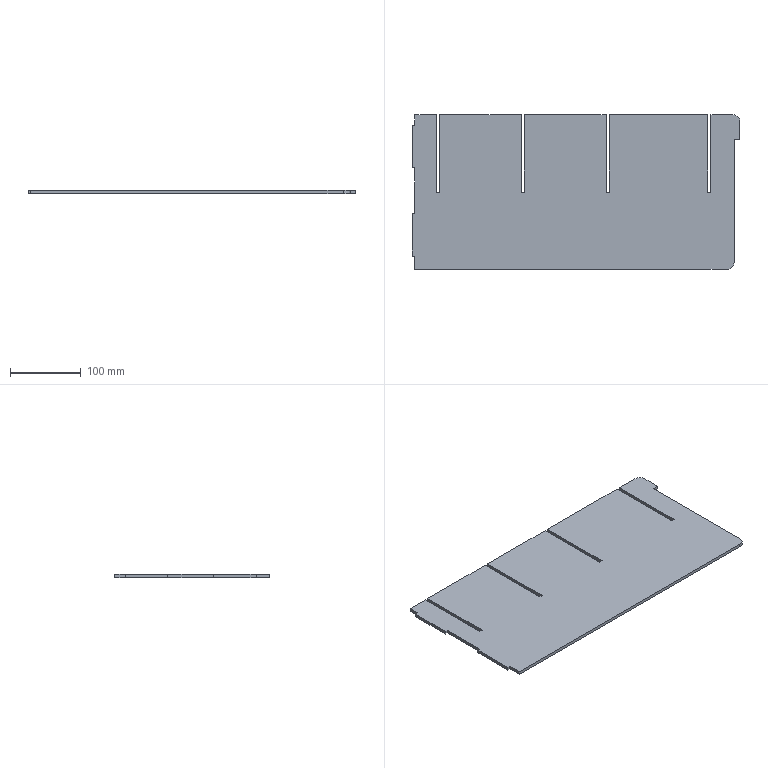Part | SolidWorks | features Fillet 1, FlatPattern 1, SMBaseFlange 1, SheetMetal 1 | 1 solid | 34 faces | box 464 x 218.7 x 4.5 mm | volume 438971 mm3 | plane 32 | cylinder 2 | commonest cylinder face diameters 20 x2
STEP:
#1=CARTESIAN_POINT('',(-230.,45.,0.));
#2=VERTEX_POINT('',#1);
#3=CARTESIAN_POINT('',(-230.,30.,0.));
#4=VERTEX_POINT('',#3);
#5=CARTESIAN_POINT('',(-230.,45.,0.));
#6=DIRECTION('',(0.,-1.,0.));
#7=VECTOR('',#6,1000.);
#8=LINE('',#5,#7);
#9=EDGE_CURVE('',#2,#4,#8,.T.);
#10=ORIENTED_EDGE('',*,*,#9,.T.);
#11=CARTESIAN_POINT('',(-230.,30.,4.5));
#12=VERTEX_POINT('',#11);
#13=CARTESIAN_POINT('',(-230.,30.,4.5));
#14=DIRECTION('',(0.,0.,-1.));
#15=VECTOR('',#14,1000.);
#16=LINE('',#13,#15);
#17=EDGE_CURVE('',#12,#4,#16,.T.);
#18=ORIENTED_EDGE('',*,*,#17,.F.);
#19=CARTESIAN_POINT('',(-230.,45.,4.5));
#20=VERTEX_POINT('',#19);
#21=CARTESIAN_POINT('',(-230.,45.,4.5));
#22=DIRECTION('',(0.,-1.,0.));
#23=VECTOR('',#22,1000.);
#24=LINE('',#21,#23);
#25=EDGE_CURVE('',#20,#12,#24,.T.);
#26=ORIENTED_EDGE('',*,*,#25,.F.);
#27=CARTESIAN_POINT('',(-230.,45.,4.5));
#28=DIRECTION('',(0.,0.,-1.));
#29=VECTOR('',#28,1000.);
#30=LINE('',#27,#29);
#31=EDGE_CURVE('',#20,#2,#30,.T.);
#32=ORIENTED_EDGE('',*,*,#31,.T.);
#33=EDGE_LOOP('',(#10,#18,#26,#32));
#34=FACE_OUTER_BOUND('',#33,.T.);
#35=CARTESIAN_POINT('',(-230.,45.,4.5));
#36=DIRECTION('',(1.,0.,0.));
#37=DIRECTION('',(0.,1.,0.));
#38=AXIS2_PLACEMENT_3D('',#35,#36,#37);
#39=PLANE('',#38);
#40=ADVANCED_FACE('',(#34),#39,.F.);
#41=CARTESIAN_POINT('',(-234.,30.,0.));
#42=VERTEX_POINT('',#41);
#43=CARTESIAN_POINT('',(-230.,30.,0.));
#44=DIRECTION('',(-1.,0.,0.));
#45=VECTOR('',#44,1000.);
#46=LINE('',#43,#45);
#47=EDGE_CURVE('',#4,#42,#46,.T.);
#48=ORIENTED_EDGE('',*,*,#47,.T.);
#49=CARTESIAN_POINT('',(-234.,30.,4.5));
#50=VERTEX_POINT('',#49);
#51=CARTESIAN_POINT('',(-234.,30.,4.5));
#52=DIRECTION('',(0.,0.,-1.));
#53=VECTOR('',#52,1000.);
#54=LINE('',#51,#53);
#55=EDGE_CURVE('',#50,#42,#54,.T.);
#56=ORIENTED_EDGE('',*,*,#55,.F.);
#57=CARTESIAN_POINT('',(-230.,30.,4.5));
#58=DIRECTION('',(-1.,0.,0.));
#59=VECTOR('',#58,1000.);
#60=LINE('',#57,#59);
#61=EDGE_CURVE('',#12,#50,#60,.T.);
#62=ORIENTED_EDGE('',*,*,#61,.F.);
#63=ORIENTED_EDGE('',*,*,#17,.T.);
#64=EDGE_LOOP('',(#48,#56,#62,#63));
#65=FACE_OUTER_BOUND('',#64,.T.);
#66=CARTESIAN_POINT('',(-230.,30.,4.5));
#67=DIRECTION('',(0.,-1.,0.));
#68=DIRECTION('',(0.,0.,-1.));
#69=AXIS2_PLACEMENT_3D('',#66,#67,#68);
#70=PLANE('',#69);
#71=ADVANCED_FACE('',(#65),#70,.F.);
#72=CARTESIAN_POINT('',(-234.,-30.,0.));
#73=VERTEX_POINT('',#72);
#74=CARTESIAN_POINT('',(-234.,30.,0.));
#75=DIRECTION('',(0.,-1.,0.));
#76=VECTOR('',#75,1000.);
#77=LINE('',#74,#76);
#78=EDGE_CURVE('',#42,#73,#77,.T.);
#79=ORIENTED_EDGE('',*,*,#78,.T.);
#80=CARTESIAN_POINT('',(-234.,-30.,4.5));
#81=VERTEX_POINT('',#80);
#82=CARTESIAN_POINT('',(-234.,-30.,4.5));
#83=DIRECTION('',(0.,0.,-1.));
#84=VECTOR('',#83,1000.);
#85=LINE('',#82,#84);
#86=EDGE_CURVE('',#81,#73,#85,.T.);
#87=ORIENTED_EDGE('',*,*,#86,.F.);
#88=CARTESIAN_POINT('',(-234.,30.,4.5));
#89=DIRECTION('',(0.,-1.,0.));
#90=VECTOR('',#89,1000.);
#91=LINE('',#88,#90);
#92=EDGE_CURVE('',#50,#81,#91,.T.);
#93=ORIENTED_EDGE('',*,*,#92,.F.);
#94=ORIENTED_EDGE('',*,*,#55,.T.);
#95=EDGE_LOOP('',(#79,#87,#93,#94));
#96=FACE_OUTER_BOUND('',#95,.T.);
#97=CARTESIAN_POINT('',(-234.,30.,4.5));
#98=DIRECTION('',(1.,0.,0.));
#99=DIRECTION('',(0.,0.,-1.));
#100=AXIS2_PLACEMENT_3D('',#97,#98,#99);
#101=PLANE('',#100);
#102=ADVANCED_FACE('',(#96),#101,.F.);
#103=CARTESIAN_POINT('',(-230.,-30.,0.));
#104=VERTEX_POINT('',#103);
#105=CARTESIAN_POINT('',(-234.,-30.,0.));
#106=DIRECTION('',(1.,0.,0.));
#107=VECTOR('',#106,1000.);
#108=LINE('',#105,#107);
#109=EDGE_CURVE('',#73,#104,#108,.T.);
#110=ORIENTED_EDGE('',*,*,#109,.T.);
#111=CARTESIAN_POINT('',(-230.,-30.,4.5));
#112=VERTEX_POINT('',#111);
#113=CARTESIAN_POINT('',(-230.,-30.,4.5));
#114=DIRECTION('',(0.,0.,-1.));
#115=VECTOR('',#114,1000.);
#116=LINE('',#113,#115);
#117=EDGE_CURVE('',#112,#104,#116,.T.);
#118=ORIENTED_EDGE('',*,*,#117,.F.);
#119=CARTESIAN_POINT('',(-234.,-30.,4.5));
#120=DIRECTION('',(1.,0.,0.));
#121=VECTOR('',#120,1000.);
#122=LINE('',#119,#121);
#123=EDGE_CURVE('',#81,#112,#122,.T.);
#124=ORIENTED_EDGE('',*,*,#123,.F.);
#125=ORIENTED_EDGE('',*,*,#86,.T.);
#126=EDGE_LOOP('',(#110,#118,#124,#125));
#127=FACE_OUTER_BOUND('',#126,.T.);
#128=CARTESIAN_POINT('',(-234.,-30.,4.5));
#129=DIRECTION('',(0.,1.,0.));
#130=DIRECTION('',(0.,0.,1.));
#131=AXIS2_PLACEMENT_3D('',#128,#129,#130);
#132=PLANE('',#131);
#133=ADVANCED_FACE('',(#127),#132,.F.);
#134=CARTESIAN_POINT('',(-230.,-95.,0.));
#135=VERTEX_POINT('',#134);
#136=CARTESIAN_POINT('',(-230.,-30.,0.));
#137=DIRECTION('',(0.,-1.,0.));
#138=VECTOR('',#137,1000.);
#139=LINE('',#136,#138);
#140=EDGE_CURVE('',#104,#135,#139,.T.);
#141=ORIENTED_EDGE('',*,*,#140,.T.);
#142=CARTESIAN_POINT('',(-230.,-95.,4.5));
#143=VERTEX_POINT('',#142);
#144=CARTESIAN_POINT('',(-230.,-95.,4.5));
#145=DIRECTION('',(0.,0.,-1.));
#146=VECTOR('',#145,1000.);
#147=LINE('',#144,#146);
#148=EDGE_CURVE('',#143,#135,#147,.T.);
#149=ORIENTED_EDGE('',*,*,#148,.F.);
#150=CARTESIAN_POINT('',(-230.,-30.,4.5));
#151=DIRECTION('',(0.,-1.,0.));
#152=VECTOR('',#151,1000.);
#153=LINE('',#150,#152);
#154=EDGE_CURVE('',#112,#143,#153,.T.);
#155=ORIENTED_EDGE('',*,*,#154,.F.);
#156=ORIENTED_EDGE('',*,*,#117,.T.);
#157=EDGE_LOOP('',(#141,#149,#155,#156));
#158=FACE_OUTER_BOUND('',#157,.T.);
#159=CARTESIAN_POINT('',(-230.,-30.,4.5));
#160=DIRECTION('',(1.,0.,0.));
#161=DIRECTION('',(0.,1.,0.));
#162=AXIS2_PLACEMENT_3D('',#159,#160,#161);
#163=PLANE('',#162);
#164=ADVANCED_FACE('',(#158),#163,.F.);
#165=CARTESIAN_POINT('',(-234.,-95.,0.));
#166=VERTEX_POINT('',#165);
#167=CARTESIAN_POINT('',(-234.,-95.,0.));
#168=DIRECTION('',(-1.,0.,0.));
#169=VECTOR('',#168,1000.);
#170=LINE('',#167,#169);
#171=EDGE_CURVE('',#135,#166,#170,.T.);
#172=ORIENTED_EDGE('',*,*,#171,.T.);
#173=CARTESIAN_POINT('',(-234.,-95.,4.5));
#174=VERTEX_POINT('',#173);
#175=CARTESIAN_POINT('',(-234.,-95.,4.5));
#176=DIRECTION('',(0.,0.,-1.));
#177=VECTOR('',#176,1000.);
#178=LINE('',#175,#177);
#179=EDGE_CURVE('',#174,#166,#178,.T.);
#180=ORIENTED_EDGE('',*,*,#179,.F.);
#181=CARTESIAN_POINT('',(-234.,-95.,4.5));
#182=DIRECTION('',(-1.,0.,0.));
#183=VECTOR('',#182,1000.);
#184=LINE('',#181,#183);
#185=EDGE_CURVE('',#143,#174,#184,.T.);
#186=ORIENTED_EDGE('',*,*,#185,.F.);
#187=ORIENTED_EDGE('',*,*,#148,.T.);
#188=EDGE_LOOP('',(#172,#180,#186,#187));
#189=FACE_OUTER_BOUND('',#188,.T.);
#190=CARTESIAN_POINT('',(-234.,-95.,4.5));
#191=DIRECTION('',(0.,-1.,0.));
#192=DIRECTION('',(0.,0.,-1.));
#193=AXIS2_PLACEMENT_3D('',#190,#191,#192);
#194=PLANE('',#193);
#195=ADVANCED_FACE('',(#189),#194,.F.);
#196=CARTESIAN_POINT('',(-234.,-155.,0.));
#197=VERTEX_POINT('',#196);
#198=CARTESIAN_POINT('',(-234.,-155.,0.));
#199=DIRECTION('',(0.,-1.,0.));
#200=VECTOR('',#199,1000.);
#201=LINE('',#198,#200);
#202=EDGE_CURVE('',#166,#197,#201,.T.);
#203=ORIENTED_EDGE('',*,*,#202,.T.);
#204=CARTESIAN_POINT('',(-234.,-155.,4.5));
#205=VERTEX_POINT('',#204);
#206=CARTESIAN_POINT('',(-234.,-155.,4.5));
#207=DIRECTION('',(0.,0.,-1.));
#208=VECTOR('',#207,1000.);
#209=LINE('',#206,#208);
#210=EDGE_CURVE('',#205,#197,#209,.T.);
#211=ORIENTED_EDGE('',*,*,#210,.F.);
#212=CARTESIAN_POINT('',(-234.,-155.,4.5));
#213=DIRECTION('',(0.,-1.,0.));
#214=VECTOR('',#213,1000.);
#215=LINE('',#212,#214);
#216=EDGE_CURVE('',#174,#205,#215,.T.);
#217=ORIENTED_EDGE('',*,*,#216,.F.);
#218=ORIENTED_EDGE('',*,*,#179,.T.);
#219=EDGE_LOOP('',(#203,#211,#217,#218));
#220=FACE_OUTER_BOUND('',#219,.T.);
#221=CARTESIAN_POINT('',(-234.,-155.,4.5));
#222=DIRECTION('',(1.,0.,0.));
#223=DIRECTION('',(0.,1.,0.));
#224=AXIS2_PLACEMENT_3D('',#221,#222,#223);
#225=PLANE('',#224);
#226=ADVANCED_FACE('',(#220),#225,.F.);
#227=CARTESIAN_POINT('',(-230.,-155.,0.));
#228=VERTEX_POINT('',#227);
#229=CARTESIAN_POINT('',(-230.,-155.,0.));
#230=DIRECTION('',(1.,0.,0.));
#231=VECTOR('',#230,1000.);
#232=LINE('',#229,#231);
#233=EDGE_CURVE('',#197,#228,#232,.T.);
#234=ORIENTED_EDGE('',*,*,#233,.T.);
#235=CARTESIAN_POINT('',(-230.,-155.,4.5));
#236=VERTEX_POINT('',#235);
#237=CARTESIAN_POINT('',(-230.,-155.,4.5));
#238=DIRECTION('',(0.,0.,-1.));
#239=VECTOR('',#238,1000.);
#240=LINE('',#237,#239);
#241=EDGE_CURVE('',#236,#228,#240,.T.);
#242=ORIENTED_EDGE('',*,*,#241,.F.);
#243=CARTESIAN_POINT('',(-230.,-155.,4.5));
#244=DIRECTION('',(1.,0.,0.));
#245=VECTOR('',#244,1000.);
#246=LINE('',#243,#245);
#247=EDGE_CURVE('',#205,#236,#246,.T.);
#248=ORIENTED_EDGE('',*,*,#247,.F.);
#249=ORIENTED_EDGE('',*,*,#210,.T.);
#250=EDGE_LOOP('',(#234,#242,#248,#249));
#251=FACE_OUTER_BOUND('',#250,.T.);
#252=CARTESIAN_POINT('',(-230.,-155.,4.5));
#253=DIRECTION('',(0.,1.,0.));
#254=DIRECTION('',(0.,0.,1.));
#255=AXIS2_PLACEMENT_3D('',#252,#253,#254);
#256=PLANE('',#255);
#257=ADVANCED_FACE('',(#251),#256,.F.);
#258=CARTESIAN_POINT('',(-230.,-173.7,0.));
#259=VERTEX_POINT('',#258);
#260=CARTESIAN_POINT('',(-230.,-155.,0.));
#261=DIRECTION('',(0.,-1.,0.));
#262=VECTOR('',#261,1000.);
#263=LINE('',#260,#262);
#264=EDGE_CURVE('',#228,#259,#263,.T.);
#265=ORIENTED_EDGE('',*,*,#264,.T.);
#266=CARTESIAN_POINT('',(-230.,-173.7,4.5));
#267=VERTEX_POINT('',#266);
#268=CARTESIAN_POINT('',(-230.,-173.7,4.5));
#269=DIRECTION('',(0.,0.,-1.));
#270=VECTOR('',#269,1000.);
#271=LINE('',#268,#270);
#272=EDGE_CURVE('',#267,#259,#271,.T.);
#273=ORIENTED_EDGE('',*,*,#272,.F.);
#274=CARTESIAN_POINT('',(-230.,-155.,4.5));
#275=DIRECTION('',(0.,-1.,0.));
#276=VECTOR('',#275,1000.);
#277=LINE('',#274,#276);
#278=EDGE_CURVE('',#236,#267,#277,.T.);
#279=ORIENTED_EDGE('',*,*,#278,.F.);
#280=ORIENTED_EDGE('',*,*,#241,.T.);
#281=EDGE_LOOP('',(#265,#273,#279,#280));
#282=FACE_OUTER_BOUND('',#281,.T.);
#283=CARTESIAN_POINT('',(-230.,-155.,4.5));
#284=DIRECTION('',(1.,0.,0.));
#285=DIRECTION('',(0.,1.,0.));
#286=AXIS2_PLACEMENT_3D('',#283,#284,#285);
#287=PLANE('',#286);
#288=ADVANCED_FACE('',(#282),#287,.F.);
#289=CARTESIAN_POINT('',(211.7,-173.7,0.));
#290=VERTEX_POINT('',#289);
#291=CARTESIAN_POINT('',(-230.,-173.7,0.));
#292=DIRECTION('',(1.,0.,0.));
#293=VECTOR('',#292,1000.);
#294=LINE('',#291,#293);
#295=EDGE_CURVE('',#259,#290,#294,.T.);
#296=ORIENTED_EDGE('',*,*,#295,.T.);
#297=CARTESIAN_POINT('',(211.7,-173.7,4.5));
#298=VERTEX_POINT('',#297);
#299=CARTESIAN_POINT('',(211.7,-173.7,4.5));
#300=DIRECTION('',(0.,0.,1.));
#301=VECTOR('',#300,1000.);
#302=LINE('',#299,#301);
#303=EDGE_CURVE('',#290,#298,#302,.T.);
#304=ORIENTED_EDGE('',*,*,#303,.T.);
#305=CARTESIAN_POINT('',(-230.,-173.7,4.5));
#306=DIRECTION('',(1.,0.,0.));
#307=VECTOR('',#306,1000.);
#308=LINE('',#305,#307);
#309=EDGE_CURVE('',#267,#298,#308,.T.);
#310=ORIENTED_EDGE('',*,*,#309,.F.);
#311=ORIENTED_EDGE('',*,*,#272,.T.);
#312=EDGE_LOOP('',(#296,#304,#310,#311));
#313=FACE_OUTER_BOUND('',#312,.T.);
#314=CARTESIAN_POINT('',(-230.,-173.7,4.5));
#315=DIRECTION('',(0.,1.,0.));
#316=DIRECTION('',(0.,0.,1.));
#317=AXIS2_PLACEMENT_3D('',#314,#315,#316);
#318=PLANE('',#317);
#319=ADVANCED_FACE('',(#313),#318,.F.);
#320=CARTESIAN_POINT('',(221.7,-163.7,4.5));
#321=VERTEX_POINT('',#320);
#322=CARTESIAN_POINT('',(221.7,9.3,4.5));
#323=VERTEX_POINT('',#322);
#324=CARTESIAN_POINT('',(221.7,9.3,4.5));
#325=DIRECTION('',(0.,1.,0.));
#326=VECTOR('',#325,1000.);
#327=LINE('',#324,#326);
#328=EDGE_CURVE('',#321,#323,#327,.T.);
#329=ORIENTED_EDGE('',*,*,#328,.F.);
#330=CARTESIAN_POINT('',(221.7,-163.7,0.));
#331=VERTEX_POINT('',#330);
#332=CARTESIAN_POINT('',(221.7,-163.7,4.5));
#333=DIRECTION('',(0.,0.,-1.));
#334=VECTOR('',#333,1000.);
#335=LINE('',#332,#334);
#336=EDGE_CURVE('',#321,#331,#335,.T.);
#337=ORIENTED_EDGE('',*,*,#336,.T.);
#338=CARTESIAN_POINT('',(221.7,9.3,0.));
#339=VERTEX_POINT('',#338);
#340=CARTESIAN_POINT('',(221.7,9.3,0.));
#341=DIRECTION('',(0.,1.,0.));
#342=VECTOR('',#341,1000.);
#343=LINE('',#340,#342);
#344=EDGE_CURVE('',#331,#339,#343,.T.);
#345=ORIENTED_EDGE('',*,*,#344,.T.);
#346=CARTESIAN_POINT('',(221.7,9.3,4.5));
#347=DIRECTION('',(0.,0.,-1.));
#348=VECTOR('',#347,1000.);
#349=LINE('',#346,#348);
#350=EDGE_CURVE('',#323,#339,#349,.T.);
#351=ORIENTED_EDGE('',*,*,#350,.F.);
#352=EDGE_LOOP('',(#329,#337,#345,#351));
#353=FACE_OUTER_BOUND('',#352,.T.);
#354=CARTESIAN_POINT('',(221.7,9.3,4.5));
#355=DIRECTION('',(-1.,0.,0.));
#356=DIRECTION('',(0.,-1.,0.));
#357=AXIS2_PLACEMENT_3D('',#354,#355,#356);
#358=PLANE('',#357);
#359=ADVANCED_FACE('',(#353),#358,.F.);
#360=CARTESIAN_POINT('',(230.,9.3,0.));
#361=VERTEX_POINT('',#360);
#362=CARTESIAN_POINT('',(221.7,9.3,0.));
#363=DIRECTION('',(1.,0.,0.));
#364=VECTOR('',#363,1000.);
#365=LINE('',#362,#364);
#366=EDGE_CURVE('',#339,#361,#365,.T.);
#367=ORIENTED_EDGE('',*,*,#366,.T.);
#368=CARTESIAN_POINT('',(230.,9.3,4.5));
#369=VERTEX_POINT('',#368);
#370=CARTESIAN_POINT('',(230.,9.3,4.5));
#371=DIRECTION('',(0.,0.,-1.));
#372=VECTOR('',#371,1000.);
#373=LINE('',#370,#372);
#374=EDGE_CURVE('',#369,#361,#373,.T.);
#375=ORIENTED_EDGE('',*,*,#374,.F.);
#376=CARTESIAN_POINT('',(221.7,9.3,4.5));
#377=DIRECTION('',(1.,0.,0.));
#378=VECTOR('',#377,1000.);
#379=LINE('',#376,#378);
#380=EDGE_CURVE('',#323,#369,#379,.T.);
#381=ORIENTED_EDGE('',*,*,#380,.F.);
#382=ORIENTED_EDGE('',*,*,#350,.T.);
#383=EDGE_LOOP('',(#367,#375,#381,#382));
#384=FACE_OUTER_BOUND('',#383,.T.);
#385=CARTESIAN_POINT('',(221.7,9.3,4.5));
#386=DIRECTION('',(0.,1.,0.));
#387=DIRECTION('',(0.,0.,1.));
#388=AXIS2_PLACEMENT_3D('',#385,#386,#387);
#389=PLANE('',#388);
#390=ADVANCED_FACE('',(#384),#389,.F.);
#391=CARTESIAN_POINT('',(230.,35.,0.));
#392=VERTEX_POINT('',#391);
#393=CARTESIAN_POINT('',(230.,9.3,0.));
#394=DIRECTION('',(0.,1.,0.));
#395=VECTOR('',#394,1000.);
#396=LINE('',#393,#395);
#397=EDGE_CURVE('',#361,#392,#396,.T.);
#398=ORIENTED_EDGE('',*,*,#397,.T.);
#399=CARTESIAN_POINT('',(230.,35.,4.5));
#400=VERTEX_POINT('',#399);
#401=CARTESIAN_POINT('',(230.,35.,4.5));
#402=DIRECTION('',(0.,0.,1.));
#403=VECTOR('',#402,1000.);
#404=LINE('',#401,#403);
#405=EDGE_CURVE('',#392,#400,#404,.T.);
#406=ORIENTED_EDGE('',*,*,#405,.T.);
#407=CARTESIAN_POINT('',(230.,9.3,4.5));
#408=DIRECTION('',(0.,1.,0.));
#409=VECTOR('',#408,1000.);
#410=LINE('',#407,#409);
#411=EDGE_CURVE('',#369,#400,#410,.T.);
#412=ORIENTED_EDGE('',*,*,#411,.F.);
#413=ORIENTED_EDGE('',*,*,#374,.T.);
#414=EDGE_LOOP('',(#398,#406,#412,#413));
#415=FACE_OUTER_BOUND('',#414,.T.);
#416=CARTESIAN_POINT('',(230.,9.3,4.5));
#417=DIRECTION('',(-1.,0.,0.));
#418=DIRECTION('',(0.,-1.,0.));
#419=AXIS2_PLACEMENT_3D('',#416,#417,#418);
#420=PLANE('',#419);
#421=ADVANCED_FACE('',(#415),#420,.F.);
#422=CARTESIAN_POINT('',(220.,45.,4.5));
#423=VERTEX_POINT('',#422);
#424=CARTESIAN_POINT('',(189.,45.,4.5));
#425=VERTEX_POINT('',#424);
#426=CARTESIAN_POINT('',(189.,45.,4.5));
#427=DIRECTION('',(-1.,0.,0.));
#428=VECTOR('',#427,1000.);
#429=LINE('',#426,#428);
#430=EDGE_CURVE('',#423,#425,#429,.T.);
#431=ORIENTED_EDGE('',*,*,#430,.F.);
#432=CARTESIAN_POINT('',(220.,45.,0.));
#433=VERTEX_POINT('',#432);
#434=CARTESIAN_POINT('',(220.,45.,4.5));
#435=DIRECTION('',(0.,0.,-1.));
#436=VECTOR('',#435,1000.);
#437=LINE('',#434,#436);
#438=EDGE_CURVE('',#423,#433,#437,.T.);
#439=ORIENTED_EDGE('',*,*,#438,.T.);
#440=CARTESIAN_POINT('',(189.,45.,0.));
#441=VERTEX_POINT('',#440);
#442=CARTESIAN_POINT('',(189.,45.,0.));
#443=DIRECTION('',(-1.,0.,0.));
#444=VECTOR('',#443,1000.);
#445=LINE('',#442,#444);
#446=EDGE_CURVE('',#433,#441,#445,.T.);
#447=ORIENTED_EDGE('',*,*,#446,.T.);
#448=CARTESIAN_POINT('',(189.,45.,4.5));
#449=DIRECTION('',(0.,0.,-1.));
#450=VECTOR('',#449,1000.);
#451=LINE('',#448,#450);
#452=EDGE_CURVE('',#425,#441,#451,.T.);
#453=ORIENTED_EDGE('',*,*,#452,.F.);
#454=EDGE_LOOP('',(#431,#439,#447,#453));
#455=FACE_OUTER_BOUND('',#454,.T.);
#456=CARTESIAN_POINT('',(189.,45.,4.5));
#457=DIRECTION('',(0.,-1.,0.));
#458=DIRECTION('',(1.,0.,0.));
#459=AXIS2_PLACEMENT_3D('',#456,#457,#458);
#460=PLANE('',#459);
#461=ADVANCED_FACE('',(#455),#460,.F.);
#462=CARTESIAN_POINT('',(189.,-64.5,0.));
#463=VERTEX_POINT('',#462);
#464=CARTESIAN_POINT('',(189.,45.,0.));
#465=DIRECTION('',(0.,-1.,0.));
#466=VECTOR('',#465,1000.);
#467=LINE('',#464,#466);
#468=EDGE_CURVE('',#441,#463,#467,.T.);
#469=ORIENTED_EDGE('',*,*,#468,.T.);
#470=CARTESIAN_POINT('',(189.,-64.5,4.5));
#471=VERTEX_POINT('',#470);
#472=CARTESIAN_POINT('',(189.,-64.5,4.5));
#473=DIRECTION('',(0.,0.,-1.));
#474=VECTOR('',#473,1000.);
#475=LINE('',#472,#474);
#476=EDGE_CURVE('',#471,#463,#475,.T.);
#477=ORIENTED_EDGE('',*,*,#476,.F.);
#478=CARTESIAN_POINT('',(189.,45.,4.5));
#479=DIRECTION('',(0.,-1.,0.));
#480=VECTOR('',#479,1000.);
#481=LINE('',#478,#480);
#482=EDGE_CURVE('',#425,#471,#481,.T.);
#483=ORIENTED_EDGE('',*,*,#482,.F.);
#484=ORIENTED_EDGE('',*,*,#452,.T.);
#485=EDGE_LOOP('',(#469,#477,#483,#484));
#486=FACE_OUTER_BOUND('',#485,.T.);
#487=CARTESIAN_POINT('',(189.,45.,4.5));
#488=DIRECTION('',(1.,0.,0.));
#489=DIRECTION('',(0.,1.,0.));
#490=AXIS2_PLACEMENT_3D('',#487,#488,#489);
#491=PLANE('',#490);
#492=ADVANCED_FACE('',(#486),#491,.F.);
#493=CARTESIAN_POINT('',(184.5,-64.5,0.));
#494=VERTEX_POINT('',#493);
#495=CARTESIAN_POINT('',(189.,-64.5,0.));
#496=DIRECTION('',(-1.,0.,0.));
#497=VECTOR('',#496,1000.);
#498=LINE('',#495,#497);
#499=EDGE_CURVE('',#463,#494,#498,.T.);
#500=ORIENTED_EDGE('',*,*,#499,.T.);
#501=CARTESIAN_POINT('',(184.5,-64.5,4.5));
#502=VERTEX_POINT('',#501);
#503=CARTESIAN_POINT('',(184.5,-64.5,4.5));
#504=DIRECTION('',(0.,0.,-1.));
#505=VECTOR('',#504,1000.);
#506=LINE('',#503,#505);
#507=EDGE_CURVE('',#502,#494,#506,.T.);
#508=ORIENTED_EDGE('',*,*,#507,.F.);
#509=CARTESIAN_POINT('',(189.,-64.5,4.5));
#510=DIRECTION('',(-1.,0.,0.));
#511=VECTOR('',#510,1000.);
#512=LINE('',#509,#511);
#513=EDGE_CURVE('',#471,#502,#512,.T.);
#514=ORIENTED_EDGE('',*,*,#513,.F.);
#515=ORIENTED_EDGE('',*,*,#476,.T.);
#516=EDGE_LOOP('',(#500,#508,#514,#515));
#517=FACE_OUTER_BOUND('',#516,.T.);
#518=CARTESIAN_POINT('',(189.,-64.5,4.5));
#519=DIRECTION('',(0.,-1.,0.));
#520=DIRECTION('',(1.,0.,0.));
#521=AXIS2_PLACEMENT_3D('',#518,#519,#520);
#522=PLANE('',#521);
#523=ADVANCED_FACE('',(#517),#522,.F.);
#524=CARTESIAN_POINT('',(184.5,45.,0.));
#525=VERTEX_POINT('',#524);
#526=CARTESIAN_POINT('',(184.5,-64.5,0.));
#527=DIRECTION('',(0.,1.,0.));
#528=VECTOR('',#527,1000.);
#529=LINE('',#526,#528);
#530=EDGE_CURVE('',#494,#525,#529,.T.);
#531=ORIENTED_EDGE('',*,*,#530,.T.);
#532=CARTESIAN_POINT('',(184.5,45.,4.5));
#533=VERTEX_POINT('',#532);
#534=CARTESIAN_POINT('',(184.5,45.,4.5));
#535=DIRECTION('',(0.,0.,-1.));
#536=VECTOR('',#535,1000.);
#537=LINE('',#534,#536);
#538=EDGE_CURVE('',#533,#525,#537,.T.);
#539=ORIENTED_EDGE('',*,*,#538,.F.);
#540=CARTESIAN_POINT('',(184.5,-64.5,4.5));
#541=DIRECTION('',(0.,1.,0.));
#542=VECTOR('',#541,1000.);
#543=LINE('',#540,#542);
#544=EDGE_CURVE('',#502,#533,#543,.T.);
#545=ORIENTED_EDGE('',*,*,#544,.F.);
#546=ORIENTED_EDGE('',*,*,#507,.T.);
#547=EDGE_LOOP('',(#531,#539,#545,#546));
#548=FACE_OUTER_BOUND('',#547,.T.);
#549=CARTESIAN_POINT('',(184.5,-64.5,4.5));
#550=DIRECTION('',(-1.,0.,0.));
#551=DIRECTION('',(0.,-1.,0.));
#552=AXIS2_PLACEMENT_3D('',#549,#550,#551);
#553=PLANE('',#552);
#554=ADVANCED_FACE('',(#548),#553,.F.);
#555=CARTESIAN_POINT('',(45.,45.,0.));
#556=VERTEX_POINT('',#555);
#557=CARTESIAN_POINT('',(45.,45.,0.));
#558=DIRECTION('',(-1.,0.,0.));
#559=VECTOR('',#558,1000.);
#560=LINE('',#557,#559);
#561=EDGE_CURVE('',#525,#556,#560,.T.);
#562=ORIENTED_EDGE('',*,*,#561,.T.);
#563=CARTESIAN_POINT('',(45.,45.,4.5));
#564=VERTEX_POINT('',#563);
#565=CARTESIAN_POINT('',(45.,45.,4.5));
#566=DIRECTION('',(0.,0.,-1.));
#567=VECTOR('',#566,1000.);
#568=LINE('',#565,#567);
#569=EDGE_CURVE('',#564,#556,#568,.T.);
#570=ORIENTED_EDGE('',*,*,#569,.F.);
#571=CARTESIAN_POINT('',(45.,45.,4.5));
#572=DIRECTION('',(-1.,0.,0.));
#573=VECTOR('',#572,1000.);
#574=LINE('',#571,#573);
#575=EDGE_CURVE('',#533,#564,#574,.T.);
#576=ORIENTED_EDGE('',*,*,#575,.F.);
#577=ORIENTED_EDGE('',*,*,#538,.T.);
#578=EDGE_LOOP('',(#562,#570,#576,#577));
#579=FACE_OUTER_BOUND('',#578,.T.);
#580=CARTESIAN_POINT('',(45.,45.,4.5));
#581=DIRECTION('',(0.,-1.,0.));
#582=DIRECTION('',(1.,0.,0.));
#583=AXIS2_PLACEMENT_3D('',#580,#581,#582);
#584=PLANE('',#583);
#585=ADVANCED_FACE('',(#579),#584,.F.);
#586=CARTESIAN_POINT('',(45.,-64.5,0.));
#587=VERTEX_POINT('',#586);
#588=CARTESIAN_POINT('',(45.,45.,0.));
#589=DIRECTION('',(0.,-1.,0.));
#590=VECTOR('',#589,1000.);
#591=LINE('',#588,#590);
#592=EDGE_CURVE('',#556,#587,#591,.T.);
#593=ORIENTED_EDGE('',*,*,#592,.T.);
#594=CARTESIAN_POINT('',(45.,-64.5,4.5));
#595=VERTEX_POINT('',#594);
#596=CARTESIAN_POINT('',(45.,-64.5,4.5));
#597=DIRECTION('',(0.,0.,-1.));
#598=VECTOR('',#597,1000.);
#599=LINE('',#596,#598);
#600=EDGE_CURVE('',#595,#587,#599,.T.);
#601=ORIENTED_EDGE('',*,*,#600,.F.);
#602=CARTESIAN_POINT('',(45.,45.,4.5));
#603=DIRECTION('',(0.,-1.,0.));
#604=VECTOR('',#603,1000.);
#605=LINE('',#602,#604);
#606=EDGE_CURVE('',#564,#595,#605,.T.);
#607=ORIENTED_EDGE('',*,*,#606,.F.);
#608=ORIENTED_EDGE('',*,*,#569,.T.);
#609=EDGE_LOOP('',(#593,#601,#607,#608));
#610=FACE_OUTER_BOUND('',#609,.T.);
#611=CARTESIAN_POINT('',(45.,45.,4.5));
#612=DIRECTION('',(1.,0.,0.));
#613=DIRECTION('',(0.,1.,0.));
#614=AXIS2_PLACEMENT_3D('',#611,#612,#613);
#615=PLANE('',#614);
#616=ADVANCED_FACE('',(#610),#615,.F.);
#617=CARTESIAN_POINT('',(40.5,-64.5,0.));
#618=VERTEX_POINT('',#617);
#619=CARTESIAN_POINT('',(45.,-64.5,0.));
#620=DIRECTION('',(-1.,0.,0.));
#621=VECTOR('',#620,1000.);
#622=LINE('',#619,#621);
#623=EDGE_CURVE('',#587,#618,#622,.T.);
#624=ORIENTED_EDGE('',*,*,#623,.T.);
#625=CARTESIAN_POINT('',(40.5,-64.5,4.5));
#626=VERTEX_POINT('',#625);
#627=CARTESIAN_POINT('',(40.5,-64.5,4.5));
#628=DIRECTION('',(0.,0.,-1.));
#629=VECTOR('',#628,1000.);
#630=LINE('',#627,#629);
#631=EDGE_CURVE('',#626,#618,#630,.T.);
#632=ORIENTED_EDGE('',*,*,#631,.F.);
#633=CARTESIAN_POINT('',(45.,-64.5,4.5));
#634=DIRECTION('',(-1.,0.,0.));
#635=VECTOR('',#634,1000.);
#636=LINE('',#633,#635);
#637=EDGE_CURVE('',#595,#626,#636,.T.);
#638=ORIENTED_EDGE('',*,*,#637,.F.);
#639=ORIENTED_EDGE('',*,*,#600,.T.);
#640=EDGE_LOOP('',(#624,#632,#638,#639));
#641=FACE_OUTER_BOUND('',#640,.T.);
#642=CARTESIAN_POINT('',(45.,-64.5,4.5));
#643=DIRECTION('',(0.,-1.,0.));
#644=DIRECTION('',(0.,0.,-1.));
#645=AXIS2_PLACEMENT_3D('',#642,#643,#644);
#646=PLANE('',#645);
#647=ADVANCED_FACE('',(#641),#646,.F.);
#648=CARTESIAN_POINT('',(40.5,45.,0.));
#649=VERTEX_POINT('',#648);
#650=CARTESIAN_POINT('',(40.5,-64.5,0.));
#651=DIRECTION('',(0.,1.,0.));
#652=VECTOR('',#651,1000.);
#653=LINE('',#650,#652);
#654=EDGE_CURVE('',#618,#649,#653,.T.);
#655=ORIENTED_EDGE('',*,*,#654,.T.);
#656=CARTESIAN_POINT('',(40.5,45.,4.5));
#657=VERTEX_POINT('',#656);
#658=CARTESIAN_POINT('',(40.5,45.,4.5));
#659=DIRECTION('',(0.,0.,-1.));
#660=VECTOR('',#659,1000.);
#661=LINE('',#658,#660);
#662=EDGE_CURVE('',#657,#649,#661,.T.);
#663=ORIENTED_EDGE('',*,*,#662,.F.);
#664=CARTESIAN_POINT('',(40.5,-64.5,4.5));
#665=DIRECTION('',(0.,1.,0.));
#666=VECTOR('',#665,1000.);
#667=LINE('',#664,#666);
#668=EDGE_CURVE('',#626,#657,#667,.T.);
#669=ORIENTED_EDGE('',*,*,#668,.F.);
#670=ORIENTED_EDGE('',*,*,#631,.T.);
#671=EDGE_LOOP('',(#655,#663,#669,#670));
#672=FACE_OUTER_BOUND('',#671,.T.);
#673=CARTESIAN_POINT('',(40.5,-64.5,4.5));
#674=DIRECTION('',(-1.,0.,0.));
#675=DIRECTION('',(0.,0.,1.));
#676=AXIS2_PLACEMENT_3D('',#673,#674,#675);
#677=PLANE('',#676);
#678=ADVANCED_FACE('',(#672),#677,.F.);
#679=CARTESIAN_POINT('',(-75.,45.,0.));
#680=VERTEX_POINT('',#679);
#681=CARTESIAN_POINT('',(-75.,45.,0.));
#682=DIRECTION('',(-1.,0.,0.));
#683=VECTOR('',#682,1000.);
#684=LINE('',#681,#683);
#685=EDGE_CURVE('',#649,#680,#684,.T.);
#686=ORIENTED_EDGE('',*,*,#685,.T.);
#687=CARTESIAN_POINT('',(-75.,45.,4.5));
#688=VERTEX_POINT('',#687);
#689=CARTESIAN_POINT('',(-75.,45.,4.5));
#690=DIRECTION('',(0.,0.,-1.));
#691=VECTOR('',#690,1000.);
#692=LINE('',#689,#691);
#693=EDGE_CURVE('',#688,#680,#692,.T.);
#694=ORIENTED_EDGE('',*,*,#693,.F.);
#695=CARTESIAN_POINT('',(-75.,45.,4.5));
#696=DIRECTION('',(-1.,0.,0.));
#697=VECTOR('',#696,1000.);
#698=LINE('',#695,#697);
#699=EDGE_CURVE('',#657,#688,#698,.T.);
#700=ORIENTED_EDGE('',*,*,#699,.F.);
#701=ORIENTED_EDGE('',*,*,#662,.T.);
#702=EDGE_LOOP('',(#686,#694,#700,#701));
#703=FACE_OUTER_BOUND('',#702,.T.);
#704=CARTESIAN_POINT('',(-75.,45.,4.5));
#705=DIRECTION('',(0.,-1.,0.));
#706=DIRECTION('',(1.,0.,0.));
#707=AXIS2_PLACEMENT_3D('',#704,#705,#706);
#708=PLANE('',#707);
#709=ADVANCED_FACE('',(#703),#708,.F.);
#710=CARTESIAN_POINT('',(-75.,-64.5,0.));
#711=VERTEX_POINT('',#710);
#712=CARTESIAN_POINT('',(-75.,45.,0.));
#713=DIRECTION('',(0.,-1.,0.));
#714=VECTOR('',#713,1000.);
#715=LINE('',#712,#714);
#716=EDGE_CURVE('',#680,#711,#715,.T.);
#717=ORIENTED_EDGE('',*,*,#716,.T.);
#718=CARTESIAN_POINT('',(-75.,-64.5,4.5));
#719=VERTEX_POINT('',#718);
#720=CARTESIAN_POINT('',(-75.,-64.5,4.5));
#721=DIRECTION('',(0.,0.,-1.));
#722=VECTOR('',#721,1000.);
#723=LINE('',#720,#722);
#724=EDGE_CURVE('',#719,#711,#723,.T.);
#725=ORIENTED_EDGE('',*,*,#724,.F.);
#726=CARTESIAN_POINT('',(-75.,45.,4.5));
#727=DIRECTION('',(0.,-1.,0.));
#728=VECTOR('',#727,1000.);
#729=LINE('',#726,#728);
#730=EDGE_CURVE('',#688,#719,#729,.T.);
#731=ORIENTED_EDGE('',*,*,#730,.F.);
#732=ORIENTED_EDGE('',*,*,#693,.T.);
#733=EDGE_LOOP('',(#717,#725,#731,#732));
#734=FACE_OUTER_BOUND('',#733,.T.);
#735=CARTESIAN_POINT('',(-75.,45.,4.5));
#736=DIRECTION('',(1.,0.,0.));
#737=DIRECTION('',(0.,1.,0.));
#738=AXIS2_PLACEMENT_3D('',#735,#736,#737);
#739=PLANE('',#738);
#740=ADVANCED_FACE('',(#734),#739,.F.);
#741=CARTESIAN_POINT('',(-79.5,-64.5,0.));
#742=VERTEX_POINT('',#741);
#743=CARTESIAN_POINT('',(-75.,-64.5,0.));
#744=DIRECTION('',(-1.,0.,0.));
#745=VECTOR('',#744,1000.);
#746=LINE('',#743,#745);
#747=EDGE_CURVE('',#711,#742,#746,.T.);
#748=ORIENTED_EDGE('',*,*,#747,.T.);
#749=CARTESIAN_POINT('',(-79.5,-64.5,4.5));
#750=VERTEX_POINT('',#749);
#751=CARTESIAN_POINT('',(-79.5,-64.5,4.5));
#752=DIRECTION('',(0.,0.,-1.));
#753=VECTOR('',#752,1000.);
#754=LINE('',#751,#753);
#755=EDGE_CURVE('',#750,#742,#754,.T.);
#756=ORIENTED_EDGE('',*,*,#755,.F.);
#757=CARTESIAN_POINT('',(-75.,-64.5,4.5));
#758=DIRECTION('',(-1.,0.,0.));
#759=VECTOR('',#758,1000.);
#760=LINE('',#757,#759);
#761=EDGE_CURVE('',#719,#750,#760,.T.);
#762=ORIENTED_EDGE('',*,*,#761,.F.);
#763=ORIENTED_EDGE('',*,*,#724,.T.);
#764=EDGE_LOOP('',(#748,#756,#762,#763));
#765=FACE_OUTER_BOUND('',#764,.T.);
#766=CARTESIAN_POINT('',(-75.,-64.5,4.5));
#767=DIRECTION('',(0.,-1.,0.));
#768=DIRECTION('',(0.,0.,-1.));
#769=AXIS2_PLACEMENT_3D('',#766,#767,#768);
#770=PLANE('',#769);
#771=ADVANCED_FACE('',(#765),#770,.F.);
#772=CARTESIAN_POINT('',(-79.5,45.,0.));
#773=VERTEX_POINT('',#772);
#774=CARTESIAN_POINT('',(-79.5,-64.5,0.));
#775=DIRECTION('',(0.,1.,0.));
#776=VECTOR('',#775,1000.);
#777=LINE('',#774,#776);
#778=EDGE_CURVE('',#742,#773,#777,.T.);
#779=ORIENTED_EDGE('',*,*,#778,.T.);
#780=CARTESIAN_POINT('',(-79.5,45.,4.5));
#781=VERTEX_POINT('',#780);
#782=CARTESIAN_POINT('',(-79.5,45.,4.5));
#783=DIRECTION('',(0.,0.,-1.));
#784=VECTOR('',#783,1000.);
#785=LINE('',#782,#784);
#786=EDGE_CURVE('',#781,#773,#785,.T.);
#787=ORIENTED_EDGE('',*,*,#786,.F.);
#788=CARTESIAN_POINT('',(-79.5,-64.5,4.5));
#789=DIRECTION('',(0.,1.,0.));
#790=VECTOR('',#789,1000.);
#791=LINE('',#788,#790);
#792=EDGE_CURVE('',#750,#781,#791,.T.);
#793=ORIENTED_EDGE('',*,*,#792,.F.);
#794=ORIENTED_EDGE('',*,*,#755,.T.);
#795=EDGE_LOOP('',(#779,#787,#793,#794));
#796=FACE_OUTER_BOUND('',#795,.T.);
#797=CARTESIAN_POINT('',(-79.5,-64.5,4.5));
#798=DIRECTION('',(-1.,0.,0.));
#799=DIRECTION('',(0.,0.,1.));
#800=AXIS2_PLACEMENT_3D('',#797,#798,#799);
#801=PLANE('',#800);
#802=ADVANCED_FACE('',(#796),#801,.F.);
#803=CARTESIAN_POINT('',(-195.,45.,0.));
#804=VERTEX_POINT('',#803);
#805=CARTESIAN_POINT('',(-195.,45.,0.));
#806=DIRECTION('',(-1.,0.,0.));
#807=VECTOR('',#806,1000.);
#808=LINE('',#805,#807);
#809=EDGE_CURVE('',#773,#804,#808,.T.);
#810=ORIENTED_EDGE('',*,*,#809,.T.);
#811=CARTESIAN_POINT('',(-195.,45.,4.5));
#812=VERTEX_POINT('',#811);
#813=CARTESIAN_POINT('',(-195.,45.,4.5));
#814=DIRECTION('',(0.,0.,-1.));
#815=VECTOR('',#814,1000.);
#816=LINE('',#813,#815);
#817=EDGE_CURVE('',#812,#804,#816,.T.);
#818=ORIENTED_EDGE('',*,*,#817,.F.);
#819=CARTESIAN_POINT('',(-195.,45.,4.5));
#820=DIRECTION('',(-1.,0.,0.));
#821=VECTOR('',#820,1000.);
#822=LINE('',#819,#821);
#823=EDGE_CURVE('',#781,#812,#822,.T.);
#824=ORIENTED_EDGE('',*,*,#823,.F.);
#825=ORIENTED_EDGE('',*,*,#786,.T.);
#826=EDGE_LOOP('',(#810,#818,#824,#825));
#827=FACE_OUTER_BOUND('',#826,.T.);
#828=CARTESIAN_POINT('',(-195.,45.,4.5));
#829=DIRECTION('',(0.,-1.,0.));
#830=DIRECTION('',(1.,0.,0.));
#831=AXIS2_PLACEMENT_3D('',#828,#829,#830);
#832=PLANE('',#831);
#833=ADVANCED_FACE('',(#827),#832,.F.);
#834=CARTESIAN_POINT('',(-195.,-64.5,0.));
#835=VERTEX_POINT('',#834);
#836=CARTESIAN_POINT('',(-195.,45.,0.));
#837=DIRECTION('',(0.,-1.,0.));
#838=VECTOR('',#837,1000.);
#839=LINE('',#836,#838);
#840=EDGE_CURVE('',#804,#835,#839,.T.);
#841=ORIENTED_EDGE('',*,*,#840,.T.);
#842=CARTESIAN_POINT('',(-195.,-64.5,4.5));
#843=VERTEX_POINT('',#842);
#844=CARTESIAN_POINT('',(-195.,-64.5,4.5));
#845=DIRECTION('',(0.,0.,-1.));
#846=VECTOR('',#845,1000.);
#847=LINE('',#844,#846);
#848=EDGE_CURVE('',#843,#835,#847,.T.);
#849=ORIENTED_EDGE('',*,*,#848,.F.);
#850=CARTESIAN_POINT('',(-195.,45.,4.5));
#851=DIRECTION('',(0.,-1.,0.));
#852=VECTOR('',#851,1000.);
#853=LINE('',#850,#852);
#854=EDGE_CURVE('',#812,#843,#853,.T.);
#855=ORIENTED_EDGE('',*,*,#854,.F.);
#856=ORIENTED_EDGE('',*,*,#817,.T.);
#857=EDGE_LOOP('',(#841,#849,#855,#856));
#858=FACE_OUTER_BOUND('',#857,.T.);
#859=CARTESIAN_POINT('',(-195.,45.,4.5));
#860=DIRECTION('',(1.,0.,0.));
#861=DIRECTION('',(0.,1.,0.));
#862=AXIS2_PLACEMENT_3D('',#859,#860,#861);
#863=PLANE('',#862);
#864=ADVANCED_FACE('',(#858),#863,.F.);
#865=CARTESIAN_POINT('',(-199.5,-64.5,0.));
#866=VERTEX_POINT('',#865);
#867=CARTESIAN_POINT('',(-195.,-64.5,0.));
#868=DIRECTION('',(-1.,0.,0.));
#869=VECTOR('',#868,1000.);
#870=LINE('',#867,#869);
#871=EDGE_CURVE('',#835,#866,#870,.T.);
#872=ORIENTED_EDGE('',*,*,#871,.T.);
#873=CARTESIAN_POINT('',(-199.5,-64.5,4.5));
#874=VERTEX_POINT('',#873);
#875=CARTESIAN_POINT('',(-199.5,-64.5,4.5));
#876=DIRECTION('',(0.,0.,-1.));
#877=VECTOR('',#876,1000.);
#878=LINE('',#875,#877);
#879=EDGE_CURVE('',#874,#866,#878,.T.);
#880=ORIENTED_EDGE('',*,*,#879,.F.);
#881=CARTESIAN_POINT('',(-195.,-64.5,4.5));
#882=DIRECTION('',(-1.,0.,0.));
#883=VECTOR('',#882,1000.);
#884=LINE('',#881,#883);
#885=EDGE_CURVE('',#843,#874,#884,.T.);
#886=ORIENTED_EDGE('',*,*,#885,.F.);
#887=ORIENTED_EDGE('',*,*,#848,.T.);
#888=EDGE_LOOP('',(#872,#880,#886,#887));
#889=FACE_OUTER_BOUND('',#888,.T.);
#890=CARTESIAN_POINT('',(-195.,-64.5,4.5));
#891=DIRECTION('',(0.,-1.,0.));
#892=DIRECTION('',(0.,0.,-1.));
#893=AXIS2_PLACEMENT_3D('',#890,#891,#892);
#894=PLANE('',#893);
#895=ADVANCED_FACE('',(#889),#894,.F.);
#896=CARTESIAN_POINT('',(-199.5,45.,0.));
#897=VERTEX_POINT('',#896);
#898=CARTESIAN_POINT('',(-199.5,-64.5,0.));
#899=DIRECTION('',(0.,1.,0.));
#900=VECTOR('',#899,1000.);
#901=LINE('',#898,#900);
#902=EDGE_CURVE('',#866,#897,#901,.T.);
#903=ORIENTED_EDGE('',*,*,#902,.T.);
#904=CARTESIAN_POINT('',(-199.5,45.,4.5));
#905=VERTEX_POINT('',#904);
#906=CARTESIAN_POINT('',(-199.5,45.,4.5));
#907=DIRECTION('',(0.,0.,-1.));
#908=VECTOR('',#907,1000.);
#909=LINE('',#906,#908);
#910=EDGE_CURVE('',#905,#897,#909,.T.);
#911=ORIENTED_EDGE('',*,*,#910,.F.);
#912=CARTESIAN_POINT('',(-199.5,-64.5,4.5));
#913=DIRECTION('',(0.,1.,0.));
#914=VECTOR('',#913,1000.);
#915=LINE('',#912,#914);
#916=EDGE_CURVE('',#874,#905,#915,.T.);
#917=ORIENTED_EDGE('',*,*,#916,.F.);
#918=ORIENTED_EDGE('',*,*,#879,.T.);
#919=EDGE_LOOP('',(#903,#911,#917,#918));
#920=FACE_OUTER_BOUND('',#919,.T.);
#921=CARTESIAN_POINT('',(-199.5,-64.5,4.5));
#922=DIRECTION('',(-1.,0.,0.));
#923=DIRECTION('',(0.,-1.,0.));
#924=AXIS2_PLACEMENT_3D('',#921,#922,#923);
#925=PLANE('',#924);
#926=ADVANCED_FACE('',(#920),#925,.F.);
#927=CARTESIAN_POINT('',(-230.,45.,0.));
#928=DIRECTION('',(-1.,0.,0.));
#929=VECTOR('',#928,1000.);
#930=LINE('',#927,#929);
#931=EDGE_CURVE('',#897,#2,#930,.T.);
#932=ORIENTED_EDGE('',*,*,#931,.T.);
#933=ORIENTED_EDGE('',*,*,#31,.F.);
#934=CARTESIAN_POINT('',(-230.,45.,4.5));
#935=DIRECTION('',(-1.,0.,0.));
#936=VECTOR('',#935,1000.);
#937=LINE('',#934,#936);
#938=EDGE_CURVE('',#905,#20,#937,.T.);
#939=ORIENTED_EDGE('',*,*,#938,.F.);
#940=ORIENTED_EDGE('',*,*,#910,.T.);
#941=EDGE_LOOP('',(#932,#933,#939,#940));
#942=FACE_OUTER_BOUND('',#941,.T.);
#943=CARTESIAN_POINT('',(-230.,45.,4.5));
#944=DIRECTION('',(0.,-1.,0.));
#945=DIRECTION('',(1.,0.,0.));
#946=AXIS2_PLACEMENT_3D('',#943,#944,#945);
#947=PLANE('',#946);
#948=ADVANCED_FACE('',(#942),#947,.F.);
#949=ORIENTED_EDGE('',*,*,#309,.T.);
#950=CARTESIAN_POINT('',(211.7,-163.7,4.5));
#951=DIRECTION('',(0.,0.,1.));
#952=DIRECTION('',(-1.,0.,0.));
#953=AXIS2_PLACEMENT_3D('',#950,#951,#952);
#954=CIRCLE('',#953,10.);
#955=EDGE_CURVE('',#298,#321,#954,.T.);
#956=ORIENTED_EDGE('',*,*,#955,.T.);
#957=ORIENTED_EDGE('',*,*,#328,.T.);
#958=ORIENTED_EDGE('',*,*,#380,.T.);
#959=ORIENTED_EDGE('',*,*,#411,.T.);
#960=CARTESIAN_POINT('',(220.,35.,4.5));
#961=DIRECTION('',(0.,0.,1.));
#962=DIRECTION('',(-1.,0.,0.));
#963=AXIS2_PLACEMENT_3D('',#960,#961,#962);
#964=CIRCLE('',#963,10.);
#965=EDGE_CURVE('',#400,#423,#964,.T.);
#966=ORIENTED_EDGE('',*,*,#965,.T.);
#967=ORIENTED_EDGE('',*,*,#430,.T.);
#968=ORIENTED_EDGE('',*,*,#482,.T.);
#969=ORIENTED_EDGE('',*,*,#513,.T.);
#970=ORIENTED_EDGE('',*,*,#544,.T.);
#971=ORIENTED_EDGE('',*,*,#575,.T.);
#972=ORIENTED_EDGE('',*,*,#606,.T.);
#973=ORIENTED_EDGE('',*,*,#637,.T.);
#974=ORIENTED_EDGE('',*,*,#668,.T.);
#975=ORIENTED_EDGE('',*,*,#699,.T.);
#976=ORIENTED_EDGE('',*,*,#730,.T.);
#977=ORIENTED_EDGE('',*,*,#761,.T.);
#978=ORIENTED_EDGE('',*,*,#792,.T.);
#979=ORIENTED_EDGE('',*,*,#823,.T.);
#980=ORIENTED_EDGE('',*,*,#854,.T.);
#981=ORIENTED_EDGE('',*,*,#885,.T.);
#982=ORIENTED_EDGE('',*,*,#916,.T.);
#983=ORIENTED_EDGE('',*,*,#938,.T.);
#984=ORIENTED_EDGE('',*,*,#25,.T.);
#985=ORIENTED_EDGE('',*,*,#61,.T.);
#986=ORIENTED_EDGE('',*,*,#92,.T.);
#987=ORIENTED_EDGE('',*,*,#123,.T.);
#988=ORIENTED_EDGE('',*,*,#154,.T.);
#989=ORIENTED_EDGE('',*,*,#185,.T.);
#990=ORIENTED_EDGE('',*,*,#216,.T.);
#991=ORIENTED_EDGE('',*,*,#247,.T.);
#992=ORIENTED_EDGE('',*,*,#278,.T.);
#993=EDGE_LOOP('',(#949,#956,#957,#958,#959,#966,#967,#968,#969,#970,#971,#972,#973,#974,#975,#976,#977,#978,#979,#980,#981,#982,#983,#984,#985,#986,#987,#988,#989,#990,#991,#992));
#994=FACE_OUTER_BOUND('',#993,.T.);
#995=CARTESIAN_POINT('',(0.,0.,4.5));
#996=DIRECTION('',(0.,0.,-1.));
#997=DIRECTION('',(-1.,0.,0.));
#998=AXIS2_PLACEMENT_3D('',#995,#996,#997);
#999=PLANE('',#998);
#1000=ADVANCED_FACE('',(#994),#999,.F.);
#1001=ORIENTED_EDGE('',*,*,#344,.F.);
#1002=CARTESIAN_POINT('',(211.7,-163.7,0.));
#1003=DIRECTION('',(0.,0.,-1.));
#1004=DIRECTION('',(-1.,0.,0.));
#1005=AXIS2_PLACEMENT_3D('',#1002,#1003,#1004);
#1006=CIRCLE('',#1005,10.);
#1007=EDGE_CURVE('',#331,#290,#1006,.T.);
#1008=ORIENTED_EDGE('',*,*,#1007,.T.);
#1009=ORIENTED_EDGE('',*,*,#295,.F.);
#1010=ORIENTED_EDGE('',*,*,#264,.F.);
#1011=ORIENTED_EDGE('',*,*,#233,.F.);
#1012=ORIENTED_EDGE('',*,*,#202,.F.);
#1013=ORIENTED_EDGE('',*,*,#171,.F.);
#1014=ORIENTED_EDGE('',*,*,#140,.F.);
#1015=ORIENTED_EDGE('',*,*,#109,.F.);
#1016=ORIENTED_EDGE('',*,*,#78,.F.);
#1017=ORIENTED_EDGE('',*,*,#47,.F.);
#1018=ORIENTED_EDGE('',*,*,#9,.F.);
#1019=ORIENTED_EDGE('',*,*,#931,.F.);
#1020=ORIENTED_EDGE('',*,*,#902,.F.);
#1021=ORIENTED_EDGE('',*,*,#871,.F.);
#1022=ORIENTED_EDGE('',*,*,#840,.F.);
#1023=ORIENTED_EDGE('',*,*,#809,.F.);
#1024=ORIENTED_EDGE('',*,*,#778,.F.);
#1025=ORIENTED_EDGE('',*,*,#747,.F.);
#1026=ORIENTED_EDGE('',*,*,#716,.F.);
#1027=ORIENTED_EDGE('',*,*,#685,.F.);
#1028=ORIENTED_EDGE('',*,*,#654,.F.);
#1029=ORIENTED_EDGE('',*,*,#623,.F.);
#1030=ORIENTED_EDGE('',*,*,#592,.F.);
#1031=ORIENTED_EDGE('',*,*,#561,.F.);
#1032=ORIENTED_EDGE('',*,*,#530,.F.);
#1033=ORIENTED_EDGE('',*,*,#499,.F.);
#1034=ORIENTED_EDGE('',*,*,#468,.F.);
#1035=ORIENTED_EDGE('',*,*,#446,.F.);
#1036=CARTESIAN_POINT('',(220.,35.,0.));
#1037=DIRECTION('',(0.,0.,-1.));
#1038=DIRECTION('',(-1.,0.,0.));
#1039=AXIS2_PLACEMENT_3D('',#1036,#1037,#1038);
#1040=CIRCLE('',#1039,10.);
#1041=EDGE_CURVE('',#433,#392,#1040,.T.);
#1042=ORIENTED_EDGE('',*,*,#1041,.T.);
#1043=ORIENTED_EDGE('',*,*,#397,.F.);
#1044=ORIENTED_EDGE('',*,*,#366,.F.);
#1045=EDGE_LOOP('',(#1001,#1008,#1009,#1010,#1011,#1012,#1013,#1014,#1015,#1016,#1017,#1018,#1019,#1020,#1021,#1022,#1023,#1024,#1025,#1026,#1027,#1028,#1029,#1030,#1031,#1032,#1033,#1034,#1035,#1042,#1043,#1044));
#1046=FACE_OUTER_BOUND('',#1045,.T.);
#1047=CARTESIAN_POINT('',(0.,0.,0.));
#1048=DIRECTION('',(0.,0.,-1.));
#1049=DIRECTION('',(-1.,0.,0.));
#1050=AXIS2_PLACEMENT_3D('',#1047,#1048,#1049);
#1051=PLANE('',#1050);
#1052=ADVANCED_FACE('',(#1046),#1051,.T.);
#1053=ORIENTED_EDGE('',*,*,#955,.F.);
#1054=ORIENTED_EDGE('',*,*,#303,.F.);
#1055=ORIENTED_EDGE('',*,*,#1007,.F.);
#1056=ORIENTED_EDGE('',*,*,#336,.F.);
#1057=EDGE_LOOP('',(#1053,#1054,#1055,#1056));
#1058=FACE_OUTER_BOUND('',#1057,.T.);
#1059=CARTESIAN_POINT('',(211.7,-163.7,4.5));
#1060=DIRECTION('',(0.,0.,-1.));
#1061=DIRECTION('',(-1.,0.,0.));
#1062=AXIS2_PLACEMENT_3D('',#1059,#1060,#1061);
#1063=CYLINDRICAL_SURFACE('',#1062,10.);
#1064=ADVANCED_FACE('',(#1058),#1063,.T.);
#1065=ORIENTED_EDGE('',*,*,#965,.F.);
#1066=ORIENTED_EDGE('',*,*,#405,.F.);
#1067=ORIENTED_EDGE('',*,*,#1041,.F.);
#1068=ORIENTED_EDGE('',*,*,#438,.F.);
#1069=EDGE_LOOP('',(#1065,#1066,#1067,#1068));
#1070=FACE_OUTER_BOUND('',#1069,.T.);
#1071=CARTESIAN_POINT('',(220.,35.,4.5));
#1072=DIRECTION('',(0.,0.,-1.));
#1073=DIRECTION('',(-1.,0.,0.));
#1074=AXIS2_PLACEMENT_3D('',#1071,#1072,#1073);
#1075=CYLINDRICAL_SURFACE('',#1074,10.);
#1076=ADVANCED_FACE('',(#1070),#1075,.T.);
#1077=CLOSED_SHELL('',(#40,#71,#102,#133,#164,#195,#226,#257,#288,#319,#359,#390,#421,#461,#492,#523,#554,#585,#616,#647,#678,#709,#740,#771,#802,#833,#864,#895,#926,#948,#1000,#1052,#1064,#1076));
#1078=MANIFOLD_SOLID_BREP('',#1077);
#1079=CARTESIAN_POINT('',(0.,0.,0.));
#1080=DIRECTION('',(0.,0.,1.));
#1081=DIRECTION('',(1.,0.,0.));
#1082=AXIS2_PLACEMENT_3D('',#1079,#1080,#1081);
#1083=(LENGTH_UNIT()NAMED_UNIT(*)SI_UNIT(.MILLI.,.METRE.));
#1084=UNCERTAINTY_MEASURE_WITH_UNIT(LENGTH_MEASURE(0.00001),#1083,'','');
#1085=(NAMED_UNIT(*)PLANE_ANGLE_UNIT()SI_UNIT($,.RADIAN.));
#1086=(NAMED_UNIT(*)SI_UNIT($,.STERADIAN.)SOLID_ANGLE_UNIT());
#1087=(GEOMETRIC_REPRESENTATION_CONTEXT(3)GLOBAL_UNCERTAINTY_ASSIGNED_CONTEXT((#1084))GLOBAL_UNIT_ASSIGNED_CONTEXT((#1083,#1085,#1086))REPRESENTATION_CONTEXT('',''));
#1088=ADVANCED_BREP_SHAPE_REPRESENTATION('',(#1078,#1082),#1087);